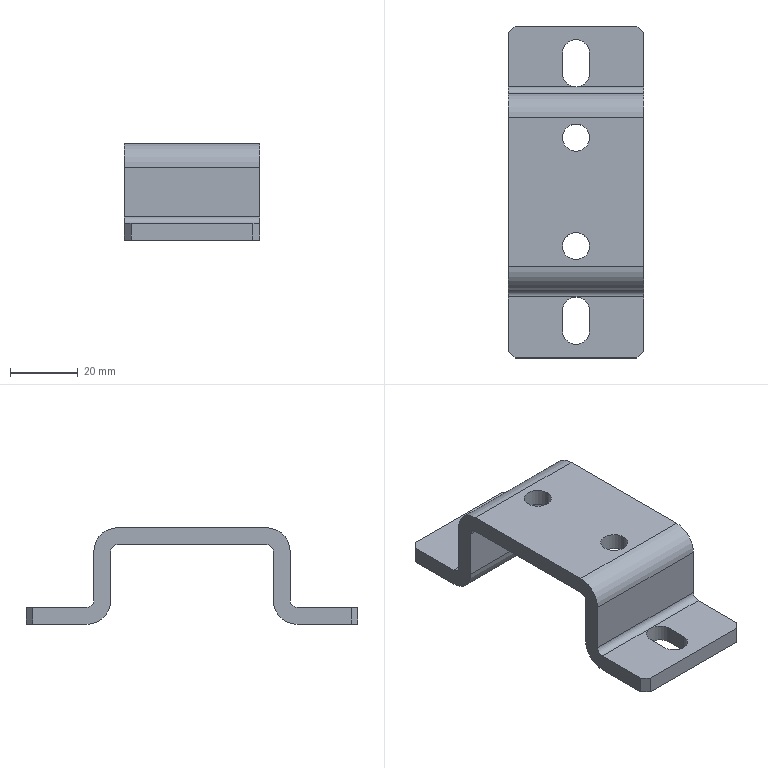Part | Creo | features DATUM PLANE 3, CURVE 2, ROUND 2, COORDINATE SYSTEM 1, CUT 1, PROTRUSION 1 | 1 solid | 38 faces | box 40 x 98 x 28.5 mm | volume 25930 mm3 | plane 22 | cylinder 16 | commonest cylinder face diameters 8 x8 4 x4 14 x4
STEP:
#1=CARTESIAN_POINT('',(0.,0.,0.));
#2=DIRECTION('',(0.,0.,1.));
#3=DIRECTION('',(1.,0.,0.));
#4=AXIS2_PLACEMENT_3D('',#1,#2,#3);
#5=CARTESIAN_POINT('',(4.,41.,0.));
#6=VERTEX_POINT('',#5);
#7=CARTESIAN_POINT('',(4.,35.,0.));
#8=VERTEX_POINT('',#7);
#9=CARTESIAN_POINT('',(4.,41.,0.));
#10=DIRECTION('',(0.,-1.,0.));
#11=VECTOR('',#10,6.);
#12=LINE('',#9,#11);
#13=EDGE_CURVE('',#6,#8,#12,.T.);
#14=ORIENTED_EDGE('',*,*,#13,.T.);
#15=CARTESIAN_POINT('',(0.,31.,0.));
#16=VERTEX_POINT('',#15);
#17=CARTESIAN_POINT('',(0.,35.,0.));
#18=DIRECTION('',(0.,0.,-1.));
#19=DIRECTION('',(1.,0.,0.));
#20=AXIS2_PLACEMENT_3D('',#17,#18,#19);
#21=CIRCLE('',#20,4.);
#22=EDGE_CURVE('',#8,#16,#21,.T.);
#23=ORIENTED_EDGE('',*,*,#22,.T.);
#24=CARTESIAN_POINT('',(20.,31.,0.));
#25=VERTEX_POINT('',#24);
#26=CARTESIAN_POINT('',(20.,31.,0.));
#27=DIRECTION('',(-1.,0.,0.));
#28=VECTOR('',#27,20.);
#29=LINE('',#26,#28);
#30=EDGE_CURVE('',#25,#16,#29,.T.);
#31=ORIENTED_EDGE('',*,*,#30,.F.);
#32=CARTESIAN_POINT('',(20.,47.,0.));
#33=VERTEX_POINT('',#32);
#34=CARTESIAN_POINT('',(20.,31.,0.));
#35=DIRECTION('',(0.,1.,0.));
#36=VECTOR('',#35,16.);
#37=LINE('',#34,#36);
#38=EDGE_CURVE('',#25,#33,#37,.T.);
#39=ORIENTED_EDGE('',*,*,#38,.T.);
#40=CARTESIAN_POINT('',(18.,49.,0.));
#41=VERTEX_POINT('',#40);
#42=CARTESIAN_POINT('',(20.,47.,0.));
#43=DIRECTION('',(-0.7071,0.7071,0.));
#44=VECTOR('',#43,2.828);
#45=LINE('',#42,#44);
#46=EDGE_CURVE('',#33,#41,#45,.T.);
#47=ORIENTED_EDGE('',*,*,#46,.T.);
#48=CARTESIAN_POINT('',(-18.,49.,0.));
#49=VERTEX_POINT('',#48);
#50=CARTESIAN_POINT('',(18.,49.,0.));
#51=DIRECTION('',(-1.,0.,0.));
#52=VECTOR('',#51,36.);
#53=LINE('',#50,#52);
#54=EDGE_CURVE('',#41,#49,#53,.T.);
#55=ORIENTED_EDGE('',*,*,#54,.T.);
#56=CARTESIAN_POINT('',(-20.,47.,0.));
#57=VERTEX_POINT('',#56);
#58=CARTESIAN_POINT('',(-18.,49.,0.));
#59=DIRECTION('',(-0.7071,-0.7071,0.));
#60=VECTOR('',#59,2.828);
#61=LINE('',#58,#60);
#62=EDGE_CURVE('',#49,#57,#61,.T.);
#63=ORIENTED_EDGE('',*,*,#62,.T.);
#64=CARTESIAN_POINT('',(-20.,31.,0.));
#65=VERTEX_POINT('',#64);
#66=CARTESIAN_POINT('',(-20.,47.,0.));
#67=DIRECTION('',(0.,-1.,0.));
#68=VECTOR('',#67,16.);
#69=LINE('',#66,#68);
#70=EDGE_CURVE('',#57,#65,#69,.T.);
#71=ORIENTED_EDGE('',*,*,#70,.T.);
#72=CARTESIAN_POINT('',(0.,31.,0.));
#73=DIRECTION('',(-1.,0.,0.));
#74=VECTOR('',#73,20.);
#75=LINE('',#72,#74);
#76=EDGE_CURVE('',#16,#65,#75,.T.);
#77=ORIENTED_EDGE('',*,*,#76,.F.);
#78=CARTESIAN_POINT('',(-4.,35.,0.));
#79=VERTEX_POINT('',#78);
#80=CARTESIAN_POINT('',(0.,35.,0.));
#81=DIRECTION('',(0.,0.,-1.));
#82=DIRECTION('',(0.,-1.,0.));
#83=AXIS2_PLACEMENT_3D('',#80,#81,#82);
#84=CIRCLE('',#83,4.);
#85=EDGE_CURVE('',#16,#79,#84,.T.);
#86=ORIENTED_EDGE('',*,*,#85,.T.);
#87=CARTESIAN_POINT('',(-4.,41.,0.));
#88=VERTEX_POINT('',#87);
#89=CARTESIAN_POINT('',(-4.,35.,0.));
#90=DIRECTION('',(0.,1.,0.));
#91=VECTOR('',#90,6.);
#92=LINE('',#89,#91);
#93=EDGE_CURVE('',#79,#88,#92,.T.);
#94=ORIENTED_EDGE('',*,*,#93,.T.);
#95=CARTESIAN_POINT('',(0.,41.,0.));
#96=DIRECTION('',(0.,0.,-1.));
#97=DIRECTION('',(-1.,0.,0.));
#98=AXIS2_PLACEMENT_3D('',#95,#96,#97);
#99=CIRCLE('',#98,4.);
#100=EDGE_CURVE('',#88,#6,#99,.T.);
#101=ORIENTED_EDGE('',*,*,#100,.T.);
#102=EDGE_LOOP('',(#14,#23,#31,#39,#47,#55,#63,#71,#77,#86,#94,#101));
#103=FACE_OUTER_BOUND('',#102,.F.);
#104=CARTESIAN_POINT('',(0.,0.,0.));
#105=DIRECTION('',(0.,0.,1.));
#106=DIRECTION('',(1.,0.,0.));
#107=AXIS2_PLACEMENT_3D('',#104,#105,#106);
#108=PLANE('',#107);
#109=ADVANCED_FACE('',(#103),#108,.F.);
#110=CARTESIAN_POINT('',(-4.,-41.,0.));
#111=VERTEX_POINT('',#110);
#112=CARTESIAN_POINT('',(-4.,-35.,0.));
#113=VERTEX_POINT('',#112);
#114=CARTESIAN_POINT('',(-4.,-41.,0.));
#115=DIRECTION('',(0.,1.,0.));
#116=VECTOR('',#115,6.);
#117=LINE('',#114,#116);
#118=EDGE_CURVE('',#111,#113,#117,.T.);
#119=ORIENTED_EDGE('',*,*,#118,.T.);
#120=CARTESIAN_POINT('',(0.,-31.,0.));
#121=VERTEX_POINT('',#120);
#122=CARTESIAN_POINT('',(0.,-35.,0.));
#123=DIRECTION('',(0.,0.,-1.));
#124=DIRECTION('',(-1.,0.,0.));
#125=AXIS2_PLACEMENT_3D('',#122,#123,#124);
#126=CIRCLE('',#125,4.);
#127=EDGE_CURVE('',#113,#121,#126,.T.);
#128=ORIENTED_EDGE('',*,*,#127,.T.);
#129=CARTESIAN_POINT('',(-20.,-31.,0.));
#130=VERTEX_POINT('',#129);
#131=CARTESIAN_POINT('',(-20.,-31.,0.));
#132=DIRECTION('',(1.,0.,0.));
#133=VECTOR('',#132,20.);
#134=LINE('',#131,#133);
#135=EDGE_CURVE('',#130,#121,#134,.T.);
#136=ORIENTED_EDGE('',*,*,#135,.F.);
#137=CARTESIAN_POINT('',(-20.,-47.,0.));
#138=VERTEX_POINT('',#137);
#139=CARTESIAN_POINT('',(-20.,-31.,0.));
#140=DIRECTION('',(0.,-1.,0.));
#141=VECTOR('',#140,16.);
#142=LINE('',#139,#141);
#143=EDGE_CURVE('',#130,#138,#142,.T.);
#144=ORIENTED_EDGE('',*,*,#143,.T.);
#145=CARTESIAN_POINT('',(-18.,-49.,0.));
#146=VERTEX_POINT('',#145);
#147=CARTESIAN_POINT('',(-20.,-47.,0.));
#148=DIRECTION('',(0.7071,-0.7071,0.));
#149=VECTOR('',#148,2.828);
#150=LINE('',#147,#149);
#151=EDGE_CURVE('',#138,#146,#150,.T.);
#152=ORIENTED_EDGE('',*,*,#151,.T.);
#153=CARTESIAN_POINT('',(18.,-49.,0.));
#154=VERTEX_POINT('',#153);
#155=CARTESIAN_POINT('',(-18.,-49.,0.));
#156=DIRECTION('',(1.,0.,0.));
#157=VECTOR('',#156,36.);
#158=LINE('',#155,#157);
#159=EDGE_CURVE('',#146,#154,#158,.T.);
#160=ORIENTED_EDGE('',*,*,#159,.T.);
#161=CARTESIAN_POINT('',(20.,-47.,0.));
#162=VERTEX_POINT('',#161);
#163=CARTESIAN_POINT('',(18.,-49.,0.));
#164=DIRECTION('',(0.7071,0.7071,0.));
#165=VECTOR('',#164,2.828);
#166=LINE('',#163,#165);
#167=EDGE_CURVE('',#154,#162,#166,.T.);
#168=ORIENTED_EDGE('',*,*,#167,.T.);
#169=CARTESIAN_POINT('',(20.,-31.,0.));
#170=VERTEX_POINT('',#169);
#171=CARTESIAN_POINT('',(20.,-47.,0.));
#172=DIRECTION('',(0.,1.,0.));
#173=VECTOR('',#172,16.);
#174=LINE('',#171,#173);
#175=EDGE_CURVE('',#162,#170,#174,.T.);
#176=ORIENTED_EDGE('',*,*,#175,.T.);
#177=CARTESIAN_POINT('',(0.,-31.,0.));
#178=DIRECTION('',(1.,0.,0.));
#179=VECTOR('',#178,20.);
#180=LINE('',#177,#179);
#181=EDGE_CURVE('',#121,#170,#180,.T.);
#182=ORIENTED_EDGE('',*,*,#181,.F.);
#183=CARTESIAN_POINT('',(4.,-35.,0.));
#184=VERTEX_POINT('',#183);
#185=CARTESIAN_POINT('',(0.,-35.,0.));
#186=DIRECTION('',(0.,0.,-1.));
#187=DIRECTION('',(0.,1.,0.));
#188=AXIS2_PLACEMENT_3D('',#185,#186,#187);
#189=CIRCLE('',#188,4.);
#190=EDGE_CURVE('',#121,#184,#189,.T.);
#191=ORIENTED_EDGE('',*,*,#190,.T.);
#192=CARTESIAN_POINT('',(4.,-41.,0.));
#193=VERTEX_POINT('',#192);
#194=CARTESIAN_POINT('',(4.,-35.,0.));
#195=DIRECTION('',(0.,-1.,0.));
#196=VECTOR('',#195,6.);
#197=LINE('',#194,#196);
#198=EDGE_CURVE('',#184,#193,#197,.T.);
#199=ORIENTED_EDGE('',*,*,#198,.T.);
#200=CARTESIAN_POINT('',(0.,-41.,0.));
#201=DIRECTION('',(0.,0.,-1.));
#202=DIRECTION('',(1.,0.,0.));
#203=AXIS2_PLACEMENT_3D('',#200,#201,#202);
#204=CIRCLE('',#203,4.);
#205=EDGE_CURVE('',#193,#111,#204,.T.);
#206=ORIENTED_EDGE('',*,*,#205,.T.);
#207=EDGE_LOOP('',(#119,#128,#136,#144,#152,#160,#168,#176,#182,#191,#199,#206));
#208=FACE_OUTER_BOUND('',#207,.F.);
#209=CARTESIAN_POINT('',(0.,0.,0.));
#210=DIRECTION('',(0.,0.,1.));
#211=DIRECTION('',(1.,0.,0.));
#212=AXIS2_PLACEMENT_3D('',#209,#210,#211);
#213=PLANE('',#212);
#214=ADVANCED_FACE('',(#208),#213,.F.);
#215=CARTESIAN_POINT('',(4.,41.,5.));
#216=VERTEX_POINT('',#215);
#217=CARTESIAN_POINT('',(4.,35.,5.));
#218=VERTEX_POINT('',#217);
#219=CARTESIAN_POINT('',(4.,41.,5.));
#220=DIRECTION('',(0.,-1.,0.));
#221=VECTOR('',#220,6.);
#222=LINE('',#219,#221);
#223=EDGE_CURVE('',#216,#218,#222,.T.);
#224=ORIENTED_EDGE('',*,*,#223,.T.);
#225=CARTESIAN_POINT('',(4.,35.,0.));
#226=DIRECTION('',(0.,0.,1.));
#227=VECTOR('',#226,5.);
#228=LINE('',#225,#227);
#229=EDGE_CURVE('',#8,#218,#228,.T.);
#230=ORIENTED_EDGE('',*,*,#229,.F.);
#231=ORIENTED_EDGE('',*,*,#13,.F.);
#232=CARTESIAN_POINT('',(4.,41.,0.));
#233=DIRECTION('',(0.,0.,1.));
#234=VECTOR('',#233,5.);
#235=LINE('',#232,#234);
#236=EDGE_CURVE('',#6,#216,#235,.T.);
#237=ORIENTED_EDGE('',*,*,#236,.T.);
#238=EDGE_LOOP('',(#224,#230,#231,#237));
#239=FACE_OUTER_BOUND('',#238,.F.);
#240=CARTESIAN_POINT('',(4.,41.,0.));
#241=DIRECTION('',(-1.,0.,0.));
#242=DIRECTION('',(0.,-1.,0.));
#243=AXIS2_PLACEMENT_3D('',#240,#241,#242);
#244=PLANE('',#243);
#245=ADVANCED_FACE('',(#239),#244,.T.);
#246=ORIENTED_EDGE('',*,*,#223,.F.);
#247=CARTESIAN_POINT('',(-4.,41.,5.));
#248=VERTEX_POINT('',#247);
#249=CARTESIAN_POINT('',(0.,41.,5.));
#250=DIRECTION('',(0.,0.,1.));
#251=DIRECTION('',(1.,0.,0.));
#252=AXIS2_PLACEMENT_3D('',#249,#250,#251);
#253=CIRCLE('',#252,4.);
#254=EDGE_CURVE('',#216,#248,#253,.T.);
#255=ORIENTED_EDGE('',*,*,#254,.T.);
#256=CARTESIAN_POINT('',(-4.,35.,5.));
#257=VERTEX_POINT('',#256);
#258=CARTESIAN_POINT('',(-4.,35.,5.));
#259=DIRECTION('',(0.,1.,0.));
#260=VECTOR('',#259,6.);
#261=LINE('',#258,#260);
#262=EDGE_CURVE('',#257,#248,#261,.T.);
#263=ORIENTED_EDGE('',*,*,#262,.F.);
#264=CARTESIAN_POINT('',(0.,31.,5.));
#265=VERTEX_POINT('',#264);
#266=CARTESIAN_POINT('',(0.,35.,5.));
#267=DIRECTION('',(0.,0.,1.));
#268=DIRECTION('',(-1.,0.,0.));
#269=AXIS2_PLACEMENT_3D('',#266,#267,#268);
#270=CIRCLE('',#269,4.);
#271=EDGE_CURVE('',#257,#265,#270,.T.);
#272=ORIENTED_EDGE('',*,*,#271,.T.);
#273=CARTESIAN_POINT('',(-20.,31.,5.));
#274=VERTEX_POINT('',#273);
#275=CARTESIAN_POINT('',(0.,31.,5.));
#276=DIRECTION('',(-1.,0.,0.));
#277=VECTOR('',#276,20.);
#278=LINE('',#275,#277);
#279=EDGE_CURVE('',#265,#274,#278,.T.);
#280=ORIENTED_EDGE('',*,*,#279,.T.);
#281=CARTESIAN_POINT('',(-20.,47.,5.));
#282=VERTEX_POINT('',#281);
#283=CARTESIAN_POINT('',(-20.,47.,5.));
#284=DIRECTION('',(0.,-1.,0.));
#285=VECTOR('',#284,16.);
#286=LINE('',#283,#285);
#287=EDGE_CURVE('',#282,#274,#286,.T.);
#288=ORIENTED_EDGE('',*,*,#287,.F.);
#289=CARTESIAN_POINT('',(-18.,49.,5.));
#290=VERTEX_POINT('',#289);
#291=CARTESIAN_POINT('',(-18.,49.,5.));
#292=DIRECTION('',(-0.7071,-0.7071,0.));
#293=VECTOR('',#292,2.828);
#294=LINE('',#291,#293);
#295=EDGE_CURVE('',#290,#282,#294,.T.);
#296=ORIENTED_EDGE('',*,*,#295,.F.);
#297=CARTESIAN_POINT('',(18.,49.,5.));
#298=VERTEX_POINT('',#297);
#299=CARTESIAN_POINT('',(18.,49.,5.));
#300=DIRECTION('',(-1.,0.,0.));
#301=VECTOR('',#300,36.);
#302=LINE('',#299,#301);
#303=EDGE_CURVE('',#298,#290,#302,.T.);
#304=ORIENTED_EDGE('',*,*,#303,.F.);
#305=CARTESIAN_POINT('',(20.,47.,5.));
#306=VERTEX_POINT('',#305);
#307=CARTESIAN_POINT('',(20.,47.,5.));
#308=DIRECTION('',(-0.7071,0.7071,0.));
#309=VECTOR('',#308,2.828);
#310=LINE('',#307,#309);
#311=EDGE_CURVE('',#306,#298,#310,.T.);
#312=ORIENTED_EDGE('',*,*,#311,.F.);
#313=CARTESIAN_POINT('',(20.,31.,5.));
#314=VERTEX_POINT('',#313);
#315=CARTESIAN_POINT('',(20.,47.,5.));
#316=DIRECTION('',(0.,-1.,0.));
#317=VECTOR('',#316,16.);
#318=LINE('',#315,#317);
#319=EDGE_CURVE('',#306,#314,#318,.T.);
#320=ORIENTED_EDGE('',*,*,#319,.T.);
#321=CARTESIAN_POINT('',(20.,31.,5.));
#322=DIRECTION('',(-1.,0.,0.));
#323=VECTOR('',#322,20.);
#324=LINE('',#321,#323);
#325=EDGE_CURVE('',#314,#265,#324,.T.);
#326=ORIENTED_EDGE('',*,*,#325,.T.);
#327=CARTESIAN_POINT('',(0.,35.,5.));
#328=DIRECTION('',(0.,0.,1.));
#329=DIRECTION('',(0.,-1.,0.));
#330=AXIS2_PLACEMENT_3D('',#327,#328,#329);
#331=CIRCLE('',#330,4.);
#332=EDGE_CURVE('',#265,#218,#331,.T.);
#333=ORIENTED_EDGE('',*,*,#332,.T.);
#334=EDGE_LOOP('',(#246,#255,#263,#272,#280,#288,#296,#304,#312,#320,#326,#333));
#335=FACE_OUTER_BOUND('',#334,.F.);
#336=CARTESIAN_POINT('',(20.,29.,5.));
#337=DIRECTION('',(0.,0.,-1.));
#338=DIRECTION('',(0.,1.,0.));
#339=AXIS2_PLACEMENT_3D('',#336,#337,#338);
#340=PLANE('',#339);
#341=ADVANCED_FACE('',(#335),#340,.F.);
#342=ORIENTED_EDGE('',*,*,#254,.F.);
#343=ORIENTED_EDGE('',*,*,#236,.F.);
#344=ORIENTED_EDGE('',*,*,#100,.F.);
#345=CARTESIAN_POINT('',(-4.,41.,0.));
#346=DIRECTION('',(0.,0.,1.));
#347=VECTOR('',#346,5.);
#348=LINE('',#345,#347);
#349=EDGE_CURVE('',#88,#248,#348,.T.);
#350=ORIENTED_EDGE('',*,*,#349,.T.);
#351=EDGE_LOOP('',(#342,#343,#344,#350));
#352=FACE_OUTER_BOUND('',#351,.F.);
#353=CARTESIAN_POINT('',(0.,41.,0.));
#354=DIRECTION('',(0.,0.,1.));
#355=DIRECTION('',(1.,0.,0.));
#356=AXIS2_PLACEMENT_3D('',#353,#354,#355);
#357=CYLINDRICAL_SURFACE('',#356,4.);
#358=ADVANCED_FACE('',(#352),#357,.F.);
#359=ORIENTED_EDGE('',*,*,#262,.T.);
#360=ORIENTED_EDGE('',*,*,#349,.F.);
#361=ORIENTED_EDGE('',*,*,#93,.F.);
#362=CARTESIAN_POINT('',(-4.,35.,0.));
#363=DIRECTION('',(0.,0.,1.));
#364=VECTOR('',#363,5.);
#365=LINE('',#362,#364);
#366=EDGE_CURVE('',#79,#257,#365,.T.);
#367=ORIENTED_EDGE('',*,*,#366,.T.);
#368=EDGE_LOOP('',(#359,#360,#361,#367));
#369=FACE_OUTER_BOUND('',#368,.F.);
#370=CARTESIAN_POINT('',(-4.,35.,0.));
#371=DIRECTION('',(1.,0.,0.));
#372=DIRECTION('',(0.,1.,0.));
#373=AXIS2_PLACEMENT_3D('',#370,#371,#372);
#374=PLANE('',#373);
#375=ADVANCED_FACE('',(#369),#374,.T.);
#376=ORIENTED_EDGE('',*,*,#271,.F.);
#377=ORIENTED_EDGE('',*,*,#366,.F.);
#378=ORIENTED_EDGE('',*,*,#85,.F.);
#379=ORIENTED_EDGE('',*,*,#22,.F.);
#380=ORIENTED_EDGE('',*,*,#229,.T.);
#381=ORIENTED_EDGE('',*,*,#332,.F.);
#382=EDGE_LOOP('',(#376,#377,#378,#379,#380,#381));
#383=FACE_OUTER_BOUND('',#382,.F.);
#384=CARTESIAN_POINT('',(0.,35.,0.));
#385=DIRECTION('',(0.,0.,1.));
#386=DIRECTION('',(1.,0.,0.));
#387=AXIS2_PLACEMENT_3D('',#384,#385,#386);
#388=CYLINDRICAL_SURFACE('',#387,4.);
#389=ADVANCED_FACE('',(#383),#388,.F.);
#390=ORIENTED_EDGE('',*,*,#325,.F.);
#391=CARTESIAN_POINT('',(20.,29.,7.));
#392=VERTEX_POINT('',#391);
#393=CARTESIAN_POINT('',(20.,31.,7.));
#394=DIRECTION('',(-1.,0.,0.));
#395=DIRECTION('',(0.,0.,-1.));
#396=AXIS2_PLACEMENT_3D('',#393,#394,#395);
#397=CIRCLE('',#396,2.);
#398=EDGE_CURVE('',#314,#392,#397,.T.);
#399=ORIENTED_EDGE('',*,*,#398,.T.);
#400=CARTESIAN_POINT('',(-20.,29.,7.));
#401=VERTEX_POINT('',#400);
#402=CARTESIAN_POINT('',(20.,29.,7.));
#403=DIRECTION('',(-1.,0.,0.));
#404=VECTOR('',#403,40.);
#405=LINE('',#402,#404);
#406=EDGE_CURVE('',#392,#401,#405,.T.);
#407=ORIENTED_EDGE('',*,*,#406,.T.);
#408=CARTESIAN_POINT('',(-20.,31.,7.));
#409=DIRECTION('',(1.,0.,0.));
#410=DIRECTION('',(0.,-1.,0.));
#411=AXIS2_PLACEMENT_3D('',#408,#409,#410);
#412=CIRCLE('',#411,2.);
#413=EDGE_CURVE('',#401,#274,#412,.T.);
#414=ORIENTED_EDGE('',*,*,#413,.T.);
#415=ORIENTED_EDGE('',*,*,#279,.F.);
#416=EDGE_LOOP('',(#390,#399,#407,#414,#415));
#417=FACE_OUTER_BOUND('',#416,.F.);
#418=CARTESIAN_POINT('',(72.144,31.,7.));
#419=DIRECTION('',(-1.,0.,0.));
#420=DIRECTION('',(0.,0.,-1.));
#421=AXIS2_PLACEMENT_3D('',#418,#419,#420);
#422=CYLINDRICAL_SURFACE('',#421,2.);
#423=ADVANCED_FACE('',(#417),#422,.F.);
#424=CARTESIAN_POINT('',(20.,-22.,28.5));
#425=VERTEX_POINT('',#424);
#426=CARTESIAN_POINT('',(20.,-29.,21.5));
#427=VERTEX_POINT('',#426);
#428=CARTESIAN_POINT('',(20.,-22.,21.5));
#429=DIRECTION('',(1.,0.,0.));
#430=DIRECTION('',(0.,0.,1.));
#431=AXIS2_PLACEMENT_3D('',#428,#429,#430);
#432=CIRCLE('',#431,7.);
#433=EDGE_CURVE('',#425,#427,#432,.T.);
#434=ORIENTED_EDGE('',*,*,#433,.F.);
#435=CARTESIAN_POINT('',(20.,22.,28.5));
#436=VERTEX_POINT('',#435);
#437=CARTESIAN_POINT('',(20.,-22.,28.5));
#438=DIRECTION('',(0.,1.,0.));
#439=VECTOR('',#438,44.);
#440=LINE('',#437,#439);
#441=EDGE_CURVE('',#425,#436,#440,.T.);
#442=ORIENTED_EDGE('',*,*,#441,.T.);
#443=CARTESIAN_POINT('',(20.,29.,21.5));
#444=VERTEX_POINT('',#443);
#445=CARTESIAN_POINT('',(20.,22.,21.5));
#446=DIRECTION('',(1.,0.,0.));
#447=DIRECTION('',(0.,1.,0.));
#448=AXIS2_PLACEMENT_3D('',#445,#446,#447);
#449=CIRCLE('',#448,7.);
#450=EDGE_CURVE('',#444,#436,#449,.T.);
#451=ORIENTED_EDGE('',*,*,#450,.F.);
#452=CARTESIAN_POINT('',(20.,29.,21.5));
#453=DIRECTION('',(0.,0.,-1.));
#454=VECTOR('',#453,14.5);
#455=LINE('',#452,#454);
#456=EDGE_CURVE('',#444,#392,#455,.T.);
#457=ORIENTED_EDGE('',*,*,#456,.T.);
#458=ORIENTED_EDGE('',*,*,#398,.F.);
#459=ORIENTED_EDGE('',*,*,#319,.F.);
#460=CARTESIAN_POINT('',(20.,47.,0.));
#461=DIRECTION('',(0.,0.,1.));
#462=VECTOR('',#461,5.);
#463=LINE('',#460,#462);
#464=EDGE_CURVE('',#33,#306,#463,.T.);
#465=ORIENTED_EDGE('',*,*,#464,.F.);
#466=ORIENTED_EDGE('',*,*,#38,.F.);
#467=CARTESIAN_POINT('',(20.,24.,7.));
#468=VERTEX_POINT('',#467);
#469=CARTESIAN_POINT('',(20.,31.,7.));
#470=DIRECTION('',(1.,0.,0.));
#471=DIRECTION('',(0.,-1.,0.));
#472=AXIS2_PLACEMENT_3D('',#469,#470,#471);
#473=CIRCLE('',#472,7.);
#474=EDGE_CURVE('',#468,#25,#473,.T.);
#475=ORIENTED_EDGE('',*,*,#474,.F.);
#476=CARTESIAN_POINT('',(20.,24.,21.5));
#477=VERTEX_POINT('',#476);
#478=CARTESIAN_POINT('',(20.,24.,7.));
#479=DIRECTION('',(0.,0.,1.));
#480=VECTOR('',#479,14.5);
#481=LINE('',#478,#480);
#482=EDGE_CURVE('',#468,#477,#481,.T.);
#483=ORIENTED_EDGE('',*,*,#482,.T.);
#484=CARTESIAN_POINT('',(20.,22.,23.5));
#485=VERTEX_POINT('',#484);
#486=CARTESIAN_POINT('',(20.,22.,21.5));
#487=DIRECTION('',(-1.,0.,0.));
#488=DIRECTION('',(0.,0.,1.));
#489=AXIS2_PLACEMENT_3D('',#486,#487,#488);
#490=CIRCLE('',#489,2.);
#491=EDGE_CURVE('',#485,#477,#490,.T.);
#492=ORIENTED_EDGE('',*,*,#491,.F.);
#493=CARTESIAN_POINT('',(20.,-22.,23.5));
#494=VERTEX_POINT('',#493);
#495=CARTESIAN_POINT('',(20.,22.,23.5));
#496=DIRECTION('',(0.,-1.,0.));
#497=VECTOR('',#496,44.);
#498=LINE('',#495,#497);
#499=EDGE_CURVE('',#485,#494,#498,.T.);
#500=ORIENTED_EDGE('',*,*,#499,.T.);
#501=CARTESIAN_POINT('',(20.,-24.,21.5));
#502=VERTEX_POINT('',#501);
#503=CARTESIAN_POINT('',(20.,-22.,21.5));
#504=DIRECTION('',(-1.,0.,0.));
#505=DIRECTION('',(0.,-1.,0.));
#506=AXIS2_PLACEMENT_3D('',#503,#504,#505);
#507=CIRCLE('',#506,2.);
#508=EDGE_CURVE('',#502,#494,#507,.T.);
#509=ORIENTED_EDGE('',*,*,#508,.F.);
#510=CARTESIAN_POINT('',(20.,-24.,7.));
#511=VERTEX_POINT('',#510);
#512=CARTESIAN_POINT('',(20.,-24.,7.));
#513=DIRECTION('',(0.,0.,1.));
#514=VECTOR('',#513,14.5);
#515=LINE('',#512,#514);
#516=EDGE_CURVE('',#511,#502,#515,.T.);
#517=ORIENTED_EDGE('',*,*,#516,.F.);
#518=CARTESIAN_POINT('',(20.,-31.,7.));
#519=DIRECTION('',(1.,0.,0.));
#520=DIRECTION('',(0.,0.,-1.));
#521=AXIS2_PLACEMENT_3D('',#518,#519,#520);
#522=CIRCLE('',#521,7.);
#523=EDGE_CURVE('',#170,#511,#522,.T.);
#524=ORIENTED_EDGE('',*,*,#523,.F.);
#525=ORIENTED_EDGE('',*,*,#175,.F.);
#526=CARTESIAN_POINT('',(20.,-47.,5.));
#527=VERTEX_POINT('',#526);
#528=CARTESIAN_POINT('',(20.,-47.,0.));
#529=DIRECTION('',(0.,0.,1.));
#530=VECTOR('',#529,5.);
#531=LINE('',#528,#530);
#532=EDGE_CURVE('',#162,#527,#531,.T.);
#533=ORIENTED_EDGE('',*,*,#532,.T.);
#534=CARTESIAN_POINT('',(20.,-31.,5.));
#535=VERTEX_POINT('',#534);
#536=CARTESIAN_POINT('',(20.,-47.,5.));
#537=DIRECTION('',(0.,1.,0.));
#538=VECTOR('',#537,16.);
#539=LINE('',#536,#538);
#540=EDGE_CURVE('',#527,#535,#539,.T.);
#541=ORIENTED_EDGE('',*,*,#540,.T.);
#542=CARTESIAN_POINT('',(20.,-29.,7.));
#543=VERTEX_POINT('',#542);
#544=CARTESIAN_POINT('',(20.,-31.,7.));
#545=DIRECTION('',(-1.,0.,0.));
#546=DIRECTION('',(0.,1.,0.));
#547=AXIS2_PLACEMENT_3D('',#544,#545,#546);
#548=CIRCLE('',#547,2.);
#549=EDGE_CURVE('',#543,#535,#548,.T.);
#550=ORIENTED_EDGE('',*,*,#549,.F.);
#551=CARTESIAN_POINT('',(20.,-29.,21.5));
#552=DIRECTION('',(0.,0.,-1.));
#553=VECTOR('',#552,14.5);
#554=LINE('',#551,#553);
#555=EDGE_CURVE('',#427,#543,#554,.T.);
#556=ORIENTED_EDGE('',*,*,#555,.F.);
#557=EDGE_LOOP('',(#434,#442,#451,#457,#458,#459,#465,#466,#475,#483,#492,#500,#509,#517,#524,#525,#533,#541,#550,#556));
#558=FACE_OUTER_BOUND('',#557,.F.);
#559=CARTESIAN_POINT('',(20.,-47.,0.));
#560=DIRECTION('',(1.,0.,0.));
#561=DIRECTION('',(0.,1.,0.));
#562=AXIS2_PLACEMENT_3D('',#559,#560,#561);
#563=PLANE('',#562);
#564=ADVANCED_FACE('',(#558),#563,.T.);
#565=ORIENTED_EDGE('',*,*,#433,.T.);
#566=CARTESIAN_POINT('',(-20.,-29.,21.5));
#567=VERTEX_POINT('',#566);
#568=CARTESIAN_POINT('',(-20.,-29.,21.5));
#569=DIRECTION('',(1.,0.,0.));
#570=VECTOR('',#569,40.);
#571=LINE('',#568,#570);
#572=EDGE_CURVE('',#567,#427,#571,.T.);
#573=ORIENTED_EDGE('',*,*,#572,.F.);
#574=CARTESIAN_POINT('',(-20.,-22.,28.5));
#575=VERTEX_POINT('',#574);
#576=CARTESIAN_POINT('',(-20.,-22.,21.5));
#577=DIRECTION('',(-1.,0.,0.));
#578=DIRECTION('',(0.,-1.,0.));
#579=AXIS2_PLACEMENT_3D('',#576,#577,#578);
#580=CIRCLE('',#579,7.);
#581=EDGE_CURVE('',#567,#575,#580,.T.);
#582=ORIENTED_EDGE('',*,*,#581,.T.);
#583=CARTESIAN_POINT('',(-20.,-22.,28.5));
#584=DIRECTION('',(1.,0.,0.));
#585=VECTOR('',#584,40.);
#586=LINE('',#583,#585);
#587=EDGE_CURVE('',#575,#425,#586,.T.);
#588=ORIENTED_EDGE('',*,*,#587,.T.);
#589=EDGE_LOOP('',(#565,#573,#582,#588));
#590=FACE_OUTER_BOUND('',#589,.F.);
#591=CARTESIAN_POINT('',(-72.144,-22.,21.5));
#592=DIRECTION('',(1.,0.,0.));
#593=DIRECTION('',(0.,0.,1.));
#594=AXIS2_PLACEMENT_3D('',#591,#592,#593);
#595=CYLINDRICAL_SURFACE('',#594,7.);
#596=ADVANCED_FACE('',(#590),#595,.T.);
#597=ORIENTED_EDGE('',*,*,#572,.T.);
#598=ORIENTED_EDGE('',*,*,#555,.T.);
#599=CARTESIAN_POINT('',(-20.,-29.,7.));
#600=VERTEX_POINT('',#599);
#601=CARTESIAN_POINT('',(20.,-29.,7.));
#602=DIRECTION('',(-1.,0.,0.));
#603=VECTOR('',#602,40.);
#604=LINE('',#601,#603);
#605=EDGE_CURVE('',#543,#600,#604,.T.);
#606=ORIENTED_EDGE('',*,*,#605,.T.);
#607=CARTESIAN_POINT('',(-20.,-29.,21.5));
#608=DIRECTION('',(0.,0.,-1.));
#609=VECTOR('',#608,14.5);
#610=LINE('',#607,#609);
#611=EDGE_CURVE('',#567,#600,#610,.T.);
#612=ORIENTED_EDGE('',*,*,#611,.F.);
#613=EDGE_LOOP('',(#597,#598,#606,#612));
#614=FACE_OUTER_BOUND('',#613,.F.);
#615=CARTESIAN_POINT('',(20.,-29.,5.));
#616=DIRECTION('',(0.,1.,0.));
#617=DIRECTION('',(0.,0.,1.));
#618=AXIS2_PLACEMENT_3D('',#615,#616,#617);
#619=PLANE('',#618);
#620=ADVANCED_FACE('',(#614),#619,.F.);
#621=ORIENTED_EDGE('',*,*,#605,.F.);
#622=ORIENTED_EDGE('',*,*,#549,.T.);
#623=CARTESIAN_POINT('',(0.,-31.,5.));
#624=VERTEX_POINT('',#623);
#625=CARTESIAN_POINT('',(20.,-31.,5.));
#626=DIRECTION('',(-1.,0.,0.));
#627=VECTOR('',#626,20.);
#628=LINE('',#625,#627);
#629=EDGE_CURVE('',#535,#624,#628,.T.);
#630=ORIENTED_EDGE('',*,*,#629,.T.);
#631=CARTESIAN_POINT('',(-20.,-31.,5.));
#632=VERTEX_POINT('',#631);
#633=CARTESIAN_POINT('',(0.,-31.,5.));
#634=DIRECTION('',(-1.,0.,0.));
#635=VECTOR('',#634,20.);
#636=LINE('',#633,#635);
#637=EDGE_CURVE('',#624,#632,#636,.T.);
#638=ORIENTED_EDGE('',*,*,#637,.T.);
#639=CARTESIAN_POINT('',(-20.,-31.,7.));
#640=DIRECTION('',(1.,0.,0.));
#641=DIRECTION('',(0.,0.,-1.));
#642=AXIS2_PLACEMENT_3D('',#639,#640,#641);
#643=CIRCLE('',#642,2.);
#644=EDGE_CURVE('',#632,#600,#643,.T.);
#645=ORIENTED_EDGE('',*,*,#644,.T.);
#646=EDGE_LOOP('',(#621,#622,#630,#638,#645));
#647=FACE_OUTER_BOUND('',#646,.F.);
#648=CARTESIAN_POINT('',(72.144,-31.,7.));
#649=DIRECTION('',(-1.,0.,0.));
#650=DIRECTION('',(0.,1.,0.));
#651=AXIS2_PLACEMENT_3D('',#648,#649,#650);
#652=CYLINDRICAL_SURFACE('',#651,2.);
#653=ADVANCED_FACE('',(#647),#652,.F.);
#654=CARTESIAN_POINT('',(-4.,-41.,5.));
#655=VERTEX_POINT('',#654);
#656=CARTESIAN_POINT('',(-4.,-35.,5.));
#657=VERTEX_POINT('',#656);
#658=CARTESIAN_POINT('',(-4.,-41.,5.));
#659=DIRECTION('',(0.,1.,0.));
#660=VECTOR('',#659,6.);
#661=LINE('',#658,#660);
#662=EDGE_CURVE('',#655,#657,#661,.T.);
#663=ORIENTED_EDGE('',*,*,#662,.F.);
#664=CARTESIAN_POINT('',(4.,-41.,5.));
#665=VERTEX_POINT('',#664);
#666=CARTESIAN_POINT('',(0.,-41.,5.));
#667=DIRECTION('',(0.,0.,1.));
#668=DIRECTION('',(-1.,0.,0.));
#669=AXIS2_PLACEMENT_3D('',#666,#667,#668);
#670=CIRCLE('',#669,4.);
#671=EDGE_CURVE('',#655,#665,#670,.T.);
#672=ORIENTED_EDGE('',*,*,#671,.T.);
#673=CARTESIAN_POINT('',(4.,-35.,5.));
#674=VERTEX_POINT('',#673);
#675=CARTESIAN_POINT('',(4.,-35.,5.));
#676=DIRECTION('',(0.,-1.,0.));
#677=VECTOR('',#676,6.);
#678=LINE('',#675,#677);
#679=EDGE_CURVE('',#674,#665,#678,.T.);
#680=ORIENTED_EDGE('',*,*,#679,.F.);
#681=CARTESIAN_POINT('',(0.,-35.,5.));
#682=DIRECTION('',(0.,0.,1.));
#683=DIRECTION('',(1.,0.,0.));
#684=AXIS2_PLACEMENT_3D('',#681,#682,#683);
#685=CIRCLE('',#684,4.);
#686=EDGE_CURVE('',#674,#624,#685,.T.);
#687=ORIENTED_EDGE('',*,*,#686,.T.);
#688=ORIENTED_EDGE('',*,*,#629,.F.);
#689=ORIENTED_EDGE('',*,*,#540,.F.);
#690=CARTESIAN_POINT('',(18.,-49.,5.));
#691=VERTEX_POINT('',#690);
#692=CARTESIAN_POINT('',(18.,-49.,5.));
#693=DIRECTION('',(0.7071,0.7071,0.));
#694=VECTOR('',#693,2.828);
#695=LINE('',#692,#694);
#696=EDGE_CURVE('',#691,#527,#695,.T.);
#697=ORIENTED_EDGE('',*,*,#696,.F.);
#698=CARTESIAN_POINT('',(-18.,-49.,5.));
#699=VERTEX_POINT('',#698);
#700=CARTESIAN_POINT('',(-18.,-49.,5.));
#701=DIRECTION('',(1.,0.,0.));
#702=VECTOR('',#701,36.);
#703=LINE('',#700,#702);
#704=EDGE_CURVE('',#699,#691,#703,.T.);
#705=ORIENTED_EDGE('',*,*,#704,.F.);
#706=CARTESIAN_POINT('',(-20.,-47.,5.));
#707=VERTEX_POINT('',#706);
#708=CARTESIAN_POINT('',(-20.,-47.,5.));
#709=DIRECTION('',(0.7071,-0.7071,0.));
#710=VECTOR('',#709,2.828);
#711=LINE('',#708,#710);
#712=EDGE_CURVE('',#707,#699,#711,.T.);
#713=ORIENTED_EDGE('',*,*,#712,.F.);
#714=CARTESIAN_POINT('',(-20.,-47.,5.));
#715=DIRECTION('',(0.,1.,0.));
#716=VECTOR('',#715,16.);
#717=LINE('',#714,#716);
#718=EDGE_CURVE('',#707,#632,#717,.T.);
#719=ORIENTED_EDGE('',*,*,#718,.T.);
#720=ORIENTED_EDGE('',*,*,#637,.F.);
#721=CARTESIAN_POINT('',(0.,-35.,5.));
#722=DIRECTION('',(0.,0.,1.));
#723=DIRECTION('',(0.,1.,0.));
#724=AXIS2_PLACEMENT_3D('',#721,#722,#723);
#725=CIRCLE('',#724,4.);
#726=EDGE_CURVE('',#624,#657,#725,.T.);
#727=ORIENTED_EDGE('',*,*,#726,.T.);
#728=EDGE_LOOP('',(#663,#672,#680,#687,#688,#689,#697,#705,#713,#719,#720,#727));
#729=FACE_OUTER_BOUND('',#728,.F.);
#730=CARTESIAN_POINT('',(20.,-49.,5.));
#731=DIRECTION('',(0.,0.,-1.));
#732=DIRECTION('',(0.,1.,0.));
#733=AXIS2_PLACEMENT_3D('',#730,#731,#732);
#734=PLANE('',#733);
#735=ADVANCED_FACE('',(#729),#734,.F.);
#736=ORIENTED_EDGE('',*,*,#662,.T.);
#737=CARTESIAN_POINT('',(-4.,-35.,0.));
#738=DIRECTION('',(0.,0.,1.));
#739=VECTOR('',#738,5.);
#740=LINE('',#737,#739);
#741=EDGE_CURVE('',#113,#657,#740,.T.);
#742=ORIENTED_EDGE('',*,*,#741,.F.);
#743=ORIENTED_EDGE('',*,*,#118,.F.);
#744=CARTESIAN_POINT('',(-4.,-41.,0.));
#745=DIRECTION('',(0.,0.,1.));
#746=VECTOR('',#745,5.);
#747=LINE('',#744,#746);
#748=EDGE_CURVE('',#111,#655,#747,.T.);
#749=ORIENTED_EDGE('',*,*,#748,.T.);
#750=EDGE_LOOP('',(#736,#742,#743,#749));
#751=FACE_OUTER_BOUND('',#750,.F.);
#752=CARTESIAN_POINT('',(-4.,-41.,0.));
#753=DIRECTION('',(1.,0.,0.));
#754=DIRECTION('',(0.,1.,0.));
#755=AXIS2_PLACEMENT_3D('',#752,#753,#754);
#756=PLANE('',#755);
#757=ADVANCED_FACE('',(#751),#756,.T.);
#758=ORIENTED_EDGE('',*,*,#686,.F.);
#759=CARTESIAN_POINT('',(4.,-35.,0.));
#760=DIRECTION('',(0.,0.,1.));
#761=VECTOR('',#760,5.);
#762=LINE('',#759,#761);
#763=EDGE_CURVE('',#184,#674,#762,.T.);
#764=ORIENTED_EDGE('',*,*,#763,.F.);
#765=ORIENTED_EDGE('',*,*,#190,.F.);
#766=ORIENTED_EDGE('',*,*,#127,.F.);
#767=ORIENTED_EDGE('',*,*,#741,.T.);
#768=ORIENTED_EDGE('',*,*,#726,.F.);
#769=EDGE_LOOP('',(#758,#764,#765,#766,#767,#768));
#770=FACE_OUTER_BOUND('',#769,.F.);
#771=CARTESIAN_POINT('',(0.,-35.,0.));
#772=DIRECTION('',(0.,0.,1.));
#773=DIRECTION('',(1.,0.,0.));
#774=AXIS2_PLACEMENT_3D('',#771,#772,#773);
#775=CYLINDRICAL_SURFACE('',#774,4.);
#776=ADVANCED_FACE('',(#770),#775,.F.);
#777=ORIENTED_EDGE('',*,*,#679,.T.);
#778=CARTESIAN_POINT('',(4.,-41.,0.));
#779=DIRECTION('',(0.,0.,1.));
#780=VECTOR('',#779,5.);
#781=LINE('',#778,#780);
#782=EDGE_CURVE('',#193,#665,#781,.T.);
#783=ORIENTED_EDGE('',*,*,#782,.F.);
#784=ORIENTED_EDGE('',*,*,#198,.F.);
#785=ORIENTED_EDGE('',*,*,#763,.T.);
#786=EDGE_LOOP('',(#777,#783,#784,#785));
#787=FACE_OUTER_BOUND('',#786,.F.);
#788=CARTESIAN_POINT('',(4.,-35.,0.));
#789=DIRECTION('',(-1.,0.,0.));
#790=DIRECTION('',(0.,-1.,0.));
#791=AXIS2_PLACEMENT_3D('',#788,#789,#790);
#792=PLANE('',#791);
#793=ADVANCED_FACE('',(#787),#792,.T.);
#794=ORIENTED_EDGE('',*,*,#671,.F.);
#795=ORIENTED_EDGE('',*,*,#748,.F.);
#796=ORIENTED_EDGE('',*,*,#205,.F.);
#797=ORIENTED_EDGE('',*,*,#782,.T.);
#798=EDGE_LOOP('',(#794,#795,#796,#797));
#799=FACE_OUTER_BOUND('',#798,.F.);
#800=CARTESIAN_POINT('',(0.,-41.,0.));
#801=DIRECTION('',(0.,0.,1.));
#802=DIRECTION('',(1.,0.,0.));
#803=AXIS2_PLACEMENT_3D('',#800,#801,#802);
#804=CYLINDRICAL_SURFACE('',#803,4.);
#805=ADVANCED_FACE('',(#799),#804,.F.);
#806=ORIENTED_EDGE('',*,*,#696,.T.);
#807=ORIENTED_EDGE('',*,*,#532,.F.);
#808=ORIENTED_EDGE('',*,*,#167,.F.);
#809=CARTESIAN_POINT('',(18.,-49.,0.));
#810=DIRECTION('',(0.,0.,1.));
#811=VECTOR('',#810,5.);
#812=LINE('',#809,#811);
#813=EDGE_CURVE('',#154,#691,#812,.T.);
#814=ORIENTED_EDGE('',*,*,#813,.T.);
#815=EDGE_LOOP('',(#806,#807,#808,#814));
#816=FACE_OUTER_BOUND('',#815,.F.);
#817=CARTESIAN_POINT('',(18.,-49.,0.));
#818=DIRECTION('',(0.7071,-0.7071,0.));
#819=DIRECTION('',(0.7071,0.7071,0.));
#820=AXIS2_PLACEMENT_3D('',#817,#818,#819);
#821=PLANE('',#820);
#822=ADVANCED_FACE('',(#816),#821,.T.);
#823=ORIENTED_EDGE('',*,*,#704,.T.);
#824=ORIENTED_EDGE('',*,*,#813,.F.);
#825=ORIENTED_EDGE('',*,*,#159,.F.);
#826=CARTESIAN_POINT('',(-18.,-49.,0.));
#827=DIRECTION('',(0.,0.,1.));
#828=VECTOR('',#827,5.);
#829=LINE('',#826,#828);
#830=EDGE_CURVE('',#146,#699,#829,.T.);
#831=ORIENTED_EDGE('',*,*,#830,.T.);
#832=EDGE_LOOP('',(#823,#824,#825,#831));
#833=FACE_OUTER_BOUND('',#832,.F.);
#834=CARTESIAN_POINT('',(-18.,-49.,0.));
#835=DIRECTION('',(0.,-1.,0.));
#836=DIRECTION('',(1.,0.,0.));
#837=AXIS2_PLACEMENT_3D('',#834,#835,#836);
#838=PLANE('',#837);
#839=ADVANCED_FACE('',(#833),#838,.T.);
#840=ORIENTED_EDGE('',*,*,#712,.T.);
#841=ORIENTED_EDGE('',*,*,#830,.F.);
#842=ORIENTED_EDGE('',*,*,#151,.F.);
#843=CARTESIAN_POINT('',(-20.,-47.,0.));
#844=DIRECTION('',(0.,0.,1.));
#845=VECTOR('',#844,5.);
#846=LINE('',#843,#845);
#847=EDGE_CURVE('',#138,#707,#846,.T.);
#848=ORIENTED_EDGE('',*,*,#847,.T.);
#849=EDGE_LOOP('',(#840,#841,#842,#848));
#850=FACE_OUTER_BOUND('',#849,.F.);
#851=CARTESIAN_POINT('',(-20.,-47.,0.));
#852=DIRECTION('',(-0.7071,-0.7071,0.));
#853=DIRECTION('',(0.7071,-0.7071,0.));
#854=AXIS2_PLACEMENT_3D('',#851,#852,#853);
#855=PLANE('',#854);
#856=ADVANCED_FACE('',(#850),#855,.T.);
#857=ORIENTED_EDGE('',*,*,#581,.F.);
#858=ORIENTED_EDGE('',*,*,#611,.T.);
#859=ORIENTED_EDGE('',*,*,#644,.F.);
#860=ORIENTED_EDGE('',*,*,#718,.F.);
#861=ORIENTED_EDGE('',*,*,#847,.F.);
#862=ORIENTED_EDGE('',*,*,#143,.F.);
#863=CARTESIAN_POINT('',(-20.,-24.,7.));
#864=VERTEX_POINT('',#863);
#865=CARTESIAN_POINT('',(-20.,-31.,7.));
#866=DIRECTION('',(-1.,0.,0.));
#867=DIRECTION('',(0.,1.,0.));
#868=AXIS2_PLACEMENT_3D('',#865,#866,#867);
#869=CIRCLE('',#868,7.);
#870=EDGE_CURVE('',#864,#130,#869,.T.);
#871=ORIENTED_EDGE('',*,*,#870,.F.);
#872=CARTESIAN_POINT('',(-20.,-24.,21.5));
#873=VERTEX_POINT('',#872);
#874=CARTESIAN_POINT('',(-20.,-24.,7.));
#875=DIRECTION('',(0.,0.,1.));
#876=VECTOR('',#875,14.5);
#877=LINE('',#874,#876);
#878=EDGE_CURVE('',#864,#873,#877,.T.);
#879=ORIENTED_EDGE('',*,*,#878,.T.);
#880=CARTESIAN_POINT('',(-20.,-22.,23.5));
#881=VERTEX_POINT('',#880);
#882=CARTESIAN_POINT('',(-20.,-22.,21.5));
#883=DIRECTION('',(1.,0.,0.));
#884=DIRECTION('',(0.,0.,1.));
#885=AXIS2_PLACEMENT_3D('',#882,#883,#884);
#886=CIRCLE('',#885,2.);
#887=EDGE_CURVE('',#881,#873,#886,.T.);
#888=ORIENTED_EDGE('',*,*,#887,.F.);
#889=CARTESIAN_POINT('',(-20.,22.,23.5));
#890=VERTEX_POINT('',#889);
#891=CARTESIAN_POINT('',(-20.,22.,23.5));
#892=DIRECTION('',(0.,-1.,0.));
#893=VECTOR('',#892,44.);
#894=LINE('',#891,#893);
#895=EDGE_CURVE('',#890,#881,#894,.T.);
#896=ORIENTED_EDGE('',*,*,#895,.F.);
#897=CARTESIAN_POINT('',(-20.,24.,21.5));
#898=VERTEX_POINT('',#897);
#899=CARTESIAN_POINT('',(-20.,22.,21.5));
#900=DIRECTION('',(1.,0.,0.));
#901=DIRECTION('',(0.,1.,0.));
#902=AXIS2_PLACEMENT_3D('',#899,#900,#901);
#903=CIRCLE('',#902,2.);
#904=EDGE_CURVE('',#898,#890,#903,.T.);
#905=ORIENTED_EDGE('',*,*,#904,.F.);
#906=CARTESIAN_POINT('',(-20.,24.,7.));
#907=VERTEX_POINT('',#906);
#908=CARTESIAN_POINT('',(-20.,24.,7.));
#909=DIRECTION('',(0.,0.,1.));
#910=VECTOR('',#909,14.5);
#911=LINE('',#908,#910);
#912=EDGE_CURVE('',#907,#898,#911,.T.);
#913=ORIENTED_EDGE('',*,*,#912,.F.);
#914=CARTESIAN_POINT('',(-20.,31.,7.));
#915=DIRECTION('',(-1.,0.,0.));
#916=DIRECTION('',(0.,0.,-1.));
#917=AXIS2_PLACEMENT_3D('',#914,#915,#916);
#918=CIRCLE('',#917,7.);
#919=EDGE_CURVE('',#65,#907,#918,.T.);
#920=ORIENTED_EDGE('',*,*,#919,.F.);
#921=ORIENTED_EDGE('',*,*,#70,.F.);
#922=CARTESIAN_POINT('',(-20.,47.,0.));
#923=DIRECTION('',(0.,0.,1.));
#924=VECTOR('',#923,5.);
#925=LINE('',#922,#924);
#926=EDGE_CURVE('',#57,#282,#925,.T.);
#927=ORIENTED_EDGE('',*,*,#926,.T.);
#928=ORIENTED_EDGE('',*,*,#287,.T.);
#929=ORIENTED_EDGE('',*,*,#413,.F.);
#930=CARTESIAN_POINT('',(-20.,29.,21.5));
#931=VERTEX_POINT('',#930);
#932=CARTESIAN_POINT('',(-20.,29.,21.5));
#933=DIRECTION('',(0.,0.,-1.));
#934=VECTOR('',#933,14.5);
#935=LINE('',#932,#934);
#936=EDGE_CURVE('',#931,#401,#935,.T.);
#937=ORIENTED_EDGE('',*,*,#936,.F.);
#938=CARTESIAN_POINT('',(-20.,22.,28.5));
#939=VERTEX_POINT('',#938);
#940=CARTESIAN_POINT('',(-20.,22.,21.5));
#941=DIRECTION('',(-1.,0.,0.));
#942=DIRECTION('',(0.,0.,1.));
#943=AXIS2_PLACEMENT_3D('',#940,#941,#942);
#944=CIRCLE('',#943,7.);
#945=EDGE_CURVE('',#939,#931,#944,.T.);
#946=ORIENTED_EDGE('',*,*,#945,.F.);
#947=CARTESIAN_POINT('',(-20.,22.,28.5));
#948=DIRECTION('',(0.,-1.,0.));
#949=VECTOR('',#948,44.);
#950=LINE('',#947,#949);
#951=EDGE_CURVE('',#939,#575,#950,.T.);
#952=ORIENTED_EDGE('',*,*,#951,.T.);
#953=EDGE_LOOP('',(#857,#858,#859,#860,#861,#862,#871,#879,#888,#896,#905,#913,#920,#921,#927,#928,#929,#937,#946,#952));
#954=FACE_OUTER_BOUND('',#953,.F.);
#955=CARTESIAN_POINT('',(-20.,47.,0.));
#956=DIRECTION('',(-1.,0.,0.));
#957=DIRECTION('',(0.,-1.,0.));
#958=AXIS2_PLACEMENT_3D('',#955,#956,#957);
#959=PLANE('',#958);
#960=ADVANCED_FACE('',(#954),#959,.T.);
#961=ORIENTED_EDGE('',*,*,#523,.T.);
#962=CARTESIAN_POINT('',(-20.,-24.,7.));
#963=DIRECTION('',(1.,0.,0.));
#964=VECTOR('',#963,40.);
#965=LINE('',#962,#964);
#966=EDGE_CURVE('',#864,#511,#965,.T.);
#967=ORIENTED_EDGE('',*,*,#966,.F.);
#968=ORIENTED_EDGE('',*,*,#870,.T.);
#969=ORIENTED_EDGE('',*,*,#135,.T.);
#970=ORIENTED_EDGE('',*,*,#181,.T.);
#971=EDGE_LOOP('',(#961,#967,#968,#969,#970));
#972=FACE_OUTER_BOUND('',#971,.F.);
#973=CARTESIAN_POINT('',(-72.144,-31.,7.));
#974=DIRECTION('',(1.,0.,0.));
#975=DIRECTION('',(0.,0.,-1.));
#976=AXIS2_PLACEMENT_3D('',#973,#974,#975);
#977=CYLINDRICAL_SURFACE('',#976,7.);
#978=ADVANCED_FACE('',(#972),#977,.T.);
#979=ORIENTED_EDGE('',*,*,#966,.T.);
#980=ORIENTED_EDGE('',*,*,#516,.T.);
#981=CARTESIAN_POINT('',(20.,-24.,21.5));
#982=DIRECTION('',(-1.,0.,0.));
#983=VECTOR('',#982,40.);
#984=LINE('',#981,#983);
#985=EDGE_CURVE('',#502,#873,#984,.T.);
#986=ORIENTED_EDGE('',*,*,#985,.T.);
#987=ORIENTED_EDGE('',*,*,#878,.F.);
#988=EDGE_LOOP('',(#979,#980,#986,#987));
#989=FACE_OUTER_BOUND('',#988,.F.);
#990=CARTESIAN_POINT('',(20.,-24.,23.5));
#991=DIRECTION('',(0.,-1.,0.));
#992=DIRECTION('',(0.,0.,-1.));
#993=AXIS2_PLACEMENT_3D('',#990,#991,#992);
#994=PLANE('',#993);
#995=ADVANCED_FACE('',(#989),#994,.F.);
#996=ORIENTED_EDGE('',*,*,#985,.F.);
#997=ORIENTED_EDGE('',*,*,#508,.T.);
#998=CARTESIAN_POINT('',(20.,-22.,23.5));
#999=DIRECTION('',(-1.,0.,0.));
#1000=VECTOR('',#999,40.);
#1001=LINE('',#998,#1000);
#1002=EDGE_CURVE('',#494,#881,#1001,.T.);
#1003=ORIENTED_EDGE('',*,*,#1002,.T.);
#1004=ORIENTED_EDGE('',*,*,#887,.T.);
#1005=EDGE_LOOP('',(#996,#997,#1003,#1004));
#1006=FACE_OUTER_BOUND('',#1005,.F.);
#1007=CARTESIAN_POINT('',(72.144,-22.,21.5));
#1008=DIRECTION('',(-1.,0.,0.));
#1009=DIRECTION('',(0.,-1.,0.));
#1010=AXIS2_PLACEMENT_3D('',#1007,#1008,#1009);
#1011=CYLINDRICAL_SURFACE('',#1010,2.);
#1012=ADVANCED_FACE('',(#1006),#1011,.F.);
#1013=ORIENTED_EDGE('',*,*,#1002,.F.);
#1014=ORIENTED_EDGE('',*,*,#499,.F.);
#1015=CARTESIAN_POINT('',(20.,22.,23.5));
#1016=DIRECTION('',(-1.,0.,0.));
#1017=VECTOR('',#1016,40.);
#1018=LINE('',#1015,#1017);
#1019=EDGE_CURVE('',#485,#890,#1018,.T.);
#1020=ORIENTED_EDGE('',*,*,#1019,.T.);
#1021=ORIENTED_EDGE('',*,*,#895,.T.);
#1022=EDGE_LOOP('',(#1013,#1014,#1020,#1021));
#1023=FACE_OUTER_BOUND('',#1022,.F.);
#1024=CARTESIAN_POINT('',(-4.,-16.,23.5));
#1025=VERTEX_POINT('',#1024);
#1026=CARTESIAN_POINT('',(4.,-16.,23.5));
#1027=VERTEX_POINT('',#1026);
#1028=CARTESIAN_POINT('',(0.,-16.,23.5));
#1029=DIRECTION('',(0.,0.,1.));
#1030=DIRECTION('',(-1.,0.,0.));
#1031=AXIS2_PLACEMENT_3D('',#1028,#1029,#1030);
#1032=CIRCLE('',#1031,4.);
#1033=EDGE_CURVE('',#1025,#1027,#1032,.T.);
#1034=ORIENTED_EDGE('',*,*,#1033,.F.);
#1035=CARTESIAN_POINT('',(0.,-16.,23.5));
#1036=DIRECTION('',(0.,0.,1.));
#1037=DIRECTION('',(1.,0.,0.));
#1038=AXIS2_PLACEMENT_3D('',#1035,#1036,#1037);
#1039=CIRCLE('',#1038,4.);
#1040=EDGE_CURVE('',#1027,#1025,#1039,.T.);
#1041=ORIENTED_EDGE('',*,*,#1040,.F.);
#1042=EDGE_LOOP('',(#1034,#1041));
#1043=FACE_BOUND('',#1042,.F.);
#1044=CARTESIAN_POINT('',(-4.,16.,23.5));
#1045=VERTEX_POINT('',#1044);
#1046=CARTESIAN_POINT('',(4.,16.,23.5));
#1047=VERTEX_POINT('',#1046);
#1048=CARTESIAN_POINT('',(0.,16.,23.5));
#1049=DIRECTION('',(0.,0.,1.));
#1050=DIRECTION('',(-1.,0.,0.));
#1051=AXIS2_PLACEMENT_3D('',#1048,#1049,#1050);
#1052=CIRCLE('',#1051,4.);
#1053=EDGE_CURVE('',#1045,#1047,#1052,.T.);
#1054=ORIENTED_EDGE('',*,*,#1053,.F.);
#1055=CARTESIAN_POINT('',(0.,16.,23.5));
#1056=DIRECTION('',(0.,0.,1.));
#1057=DIRECTION('',(1.,0.,0.));
#1058=AXIS2_PLACEMENT_3D('',#1055,#1056,#1057);
#1059=CIRCLE('',#1058,4.);
#1060=EDGE_CURVE('',#1047,#1045,#1059,.T.);
#1061=ORIENTED_EDGE('',*,*,#1060,.F.);
#1062=EDGE_LOOP('',(#1054,#1061));
#1063=FACE_BOUND('',#1062,.F.);
#1064=CARTESIAN_POINT('',(20.,24.,23.5));
#1065=DIRECTION('',(0.,0.,1.));
#1066=DIRECTION('',(0.,-1.,0.));
#1067=AXIS2_PLACEMENT_3D('',#1064,#1065,#1066);
#1068=PLANE('',#1067);
#1069=ADVANCED_FACE('',(#1023,#1043,#1063),#1068,.F.);
#1070=ORIENTED_EDGE('',*,*,#1053,.T.);
#1071=CARTESIAN_POINT('',(4.,16.,28.5));
#1072=VERTEX_POINT('',#1071);
#1073=CARTESIAN_POINT('',(4.,16.,23.5));
#1074=DIRECTION('',(0.,0.,1.));
#1075=VECTOR('',#1074,5.);
#1076=LINE('',#1073,#1075);
#1077=EDGE_CURVE('',#1047,#1072,#1076,.T.);
#1078=ORIENTED_EDGE('',*,*,#1077,.T.);
#1079=CARTESIAN_POINT('',(-4.,16.,28.5));
#1080=VERTEX_POINT('',#1079);
#1081=CARTESIAN_POINT('',(0.,16.,28.5));
#1082=DIRECTION('',(0.,0.,-1.));
#1083=DIRECTION('',(1.,0.,0.));
#1084=AXIS2_PLACEMENT_3D('',#1081,#1082,#1083);
#1085=CIRCLE('',#1084,4.);
#1086=EDGE_CURVE('',#1072,#1080,#1085,.T.);
#1087=ORIENTED_EDGE('',*,*,#1086,.T.);
#1088=CARTESIAN_POINT('',(-4.,16.,23.5));
#1089=DIRECTION('',(0.,0.,1.));
#1090=VECTOR('',#1089,5.);
#1091=LINE('',#1088,#1090);
#1092=EDGE_CURVE('',#1045,#1080,#1091,.T.);
#1093=ORIENTED_EDGE('',*,*,#1092,.F.);
#1094=EDGE_LOOP('',(#1070,#1078,#1087,#1093));
#1095=FACE_OUTER_BOUND('',#1094,.F.);
#1096=CARTESIAN_POINT('',(0.,16.,0.));
#1097=DIRECTION('',(0.,0.,1.));
#1098=DIRECTION('',(1.,0.,0.));
#1099=AXIS2_PLACEMENT_3D('',#1096,#1097,#1098);
#1100=CYLINDRICAL_SURFACE('',#1099,4.);
#1101=ADVANCED_FACE('',(#1095),#1100,.F.);
#1102=ORIENTED_EDGE('',*,*,#1060,.T.);
#1103=ORIENTED_EDGE('',*,*,#1092,.T.);
#1104=CARTESIAN_POINT('',(0.,16.,28.5));
#1105=DIRECTION('',(0.,0.,-1.));
#1106=DIRECTION('',(-1.,0.,0.));
#1107=AXIS2_PLACEMENT_3D('',#1104,#1105,#1106);
#1108=CIRCLE('',#1107,4.);
#1109=EDGE_CURVE('',#1080,#1072,#1108,.T.);
#1110=ORIENTED_EDGE('',*,*,#1109,.T.);
#1111=ORIENTED_EDGE('',*,*,#1077,.F.);
#1112=EDGE_LOOP('',(#1102,#1103,#1110,#1111));
#1113=FACE_OUTER_BOUND('',#1112,.F.);
#1114=CARTESIAN_POINT('',(0.,16.,0.));
#1115=DIRECTION('',(0.,0.,1.));
#1116=DIRECTION('',(1.,0.,0.));
#1117=AXIS2_PLACEMENT_3D('',#1114,#1115,#1116);
#1118=CYLINDRICAL_SURFACE('',#1117,4.);
#1119=ADVANCED_FACE('',(#1113),#1118,.F.);
#1120=ORIENTED_EDGE('',*,*,#587,.F.);
#1121=ORIENTED_EDGE('',*,*,#951,.F.);
#1122=CARTESIAN_POINT('',(20.,22.,28.5));
#1123=DIRECTION('',(-1.,0.,0.));
#1124=VECTOR('',#1123,40.);
#1125=LINE('',#1122,#1124);
#1126=EDGE_CURVE('',#436,#939,#1125,.T.);
#1127=ORIENTED_EDGE('',*,*,#1126,.F.);
#1128=ORIENTED_EDGE('',*,*,#441,.F.);
#1129=EDGE_LOOP('',(#1120,#1121,#1127,#1128));
#1130=FACE_OUTER_BOUND('',#1129,.F.);
#1131=CARTESIAN_POINT('',(4.,-16.,28.5));
#1132=VERTEX_POINT('',#1131);
#1133=CARTESIAN_POINT('',(-4.,-16.,28.5));
#1134=VERTEX_POINT('',#1133);
#1135=CARTESIAN_POINT('',(0.,-16.,28.5));
#1136=DIRECTION('',(0.,0.,-1.));
#1137=DIRECTION('',(1.,0.,0.));
#1138=AXIS2_PLACEMENT_3D('',#1135,#1136,#1137);
#1139=CIRCLE('',#1138,4.);
#1140=EDGE_CURVE('',#1132,#1134,#1139,.T.);
#1141=ORIENTED_EDGE('',*,*,#1140,.F.);
#1142=CARTESIAN_POINT('',(0.,-16.,28.5));
#1143=DIRECTION('',(0.,0.,-1.));
#1144=DIRECTION('',(-1.,0.,0.));
#1145=AXIS2_PLACEMENT_3D('',#1142,#1143,#1144);
#1146=CIRCLE('',#1145,4.);
#1147=EDGE_CURVE('',#1134,#1132,#1146,.T.);
#1148=ORIENTED_EDGE('',*,*,#1147,.F.);
#1149=EDGE_LOOP('',(#1141,#1148));
#1150=FACE_BOUND('',#1149,.F.);
#1151=ORIENTED_EDGE('',*,*,#1086,.F.);
#1152=ORIENTED_EDGE('',*,*,#1109,.F.);
#1153=EDGE_LOOP('',(#1151,#1152));
#1154=FACE_BOUND('',#1153,.F.);
#1155=CARTESIAN_POINT('',(0.,0.,28.5));
#1156=DIRECTION('',(0.,0.,1.));
#1157=DIRECTION('',(1.,0.,0.));
#1158=AXIS2_PLACEMENT_3D('',#1155,#1156,#1157);
#1159=PLANE('',#1158);
#1160=ADVANCED_FACE('',(#1130,#1150,#1154),#1159,.T.);
#1161=ORIENTED_EDGE('',*,*,#1033,.T.);
#1162=CARTESIAN_POINT('',(4.,-16.,23.5));
#1163=DIRECTION('',(0.,0.,1.));
#1164=VECTOR('',#1163,5.);
#1165=LINE('',#1162,#1164);
#1166=EDGE_CURVE('',#1027,#1132,#1165,.T.);
#1167=ORIENTED_EDGE('',*,*,#1166,.T.);
#1168=ORIENTED_EDGE('',*,*,#1140,.T.);
#1169=CARTESIAN_POINT('',(-4.,-16.,23.5));
#1170=DIRECTION('',(0.,0.,1.));
#1171=VECTOR('',#1170,5.);
#1172=LINE('',#1169,#1171);
#1173=EDGE_CURVE('',#1025,#1134,#1172,.T.);
#1174=ORIENTED_EDGE('',*,*,#1173,.F.);
#1175=EDGE_LOOP('',(#1161,#1167,#1168,#1174));
#1176=FACE_OUTER_BOUND('',#1175,.F.);
#1177=CARTESIAN_POINT('',(0.,-16.,0.));
#1178=DIRECTION('',(0.,0.,1.));
#1179=DIRECTION('',(1.,0.,0.));
#1180=AXIS2_PLACEMENT_3D('',#1177,#1178,#1179);
#1181=CYLINDRICAL_SURFACE('',#1180,4.);
#1182=ADVANCED_FACE('',(#1176),#1181,.F.);
#1183=ORIENTED_EDGE('',*,*,#1040,.T.);
#1184=ORIENTED_EDGE('',*,*,#1173,.T.);
#1185=ORIENTED_EDGE('',*,*,#1147,.T.);
#1186=ORIENTED_EDGE('',*,*,#1166,.F.);
#1187=EDGE_LOOP('',(#1183,#1184,#1185,#1186));
#1188=FACE_OUTER_BOUND('',#1187,.F.);
#1189=CARTESIAN_POINT('',(0.,-16.,0.));
#1190=DIRECTION('',(0.,0.,1.));
#1191=DIRECTION('',(1.,0.,0.));
#1192=AXIS2_PLACEMENT_3D('',#1189,#1190,#1191);
#1193=CYLINDRICAL_SURFACE('',#1192,4.);
#1194=ADVANCED_FACE('',(#1188),#1193,.F.);
#1195=ORIENTED_EDGE('',*,*,#945,.T.);
#1196=CARTESIAN_POINT('',(20.,29.,21.5));
#1197=DIRECTION('',(-1.,0.,0.));
#1198=VECTOR('',#1197,40.);
#1199=LINE('',#1196,#1198);
#1200=EDGE_CURVE('',#444,#931,#1199,.T.);
#1201=ORIENTED_EDGE('',*,*,#1200,.F.);
#1202=ORIENTED_EDGE('',*,*,#450,.T.);
#1203=ORIENTED_EDGE('',*,*,#1126,.T.);
#1204=EDGE_LOOP('',(#1195,#1201,#1202,#1203));
#1205=FACE_OUTER_BOUND('',#1204,.F.);
#1206=CARTESIAN_POINT('',(72.144,22.,21.5));
#1207=DIRECTION('',(-1.,0.,0.));
#1208=DIRECTION('',(0.,0.,1.));
#1209=AXIS2_PLACEMENT_3D('',#1206,#1207,#1208);
#1210=CYLINDRICAL_SURFACE('',#1209,7.);
#1211=ADVANCED_FACE('',(#1205),#1210,.T.);
#1212=ORIENTED_EDGE('',*,*,#1200,.T.);
#1213=ORIENTED_EDGE('',*,*,#936,.T.);
#1214=ORIENTED_EDGE('',*,*,#406,.F.);
#1215=ORIENTED_EDGE('',*,*,#456,.F.);
#1216=EDGE_LOOP('',(#1212,#1213,#1214,#1215));
#1217=FACE_OUTER_BOUND('',#1216,.F.);
#1218=CARTESIAN_POINT('',(20.,29.,28.5));
#1219=DIRECTION('',(0.,-1.,0.));
#1220=DIRECTION('',(0.,0.,-1.));
#1221=AXIS2_PLACEMENT_3D('',#1218,#1219,#1220);
#1222=PLANE('',#1221);
#1223=ADVANCED_FACE('',(#1217),#1222,.F.);
#1224=ORIENTED_EDGE('',*,*,#1019,.F.);
#1225=ORIENTED_EDGE('',*,*,#491,.T.);
#1226=CARTESIAN_POINT('',(20.,24.,21.5));
#1227=DIRECTION('',(-1.,0.,0.));
#1228=VECTOR('',#1227,40.);
#1229=LINE('',#1226,#1228);
#1230=EDGE_CURVE('',#477,#898,#1229,.T.);
#1231=ORIENTED_EDGE('',*,*,#1230,.T.);
#1232=ORIENTED_EDGE('',*,*,#904,.T.);
#1233=EDGE_LOOP('',(#1224,#1225,#1231,#1232));
#1234=FACE_OUTER_BOUND('',#1233,.F.);
#1235=CARTESIAN_POINT('',(72.144,22.,21.5));
#1236=DIRECTION('',(-1.,0.,0.));
#1237=DIRECTION('',(0.,0.,1.));
#1238=AXIS2_PLACEMENT_3D('',#1235,#1236,#1237);
#1239=CYLINDRICAL_SURFACE('',#1238,2.);
#1240=ADVANCED_FACE('',(#1234),#1239,.F.);
#1241=CARTESIAN_POINT('',(20.,24.,7.));
#1242=DIRECTION('',(-1.,0.,0.));
#1243=VECTOR('',#1242,40.);
#1244=LINE('',#1241,#1243);
#1245=EDGE_CURVE('',#468,#907,#1244,.T.);
#1246=ORIENTED_EDGE('',*,*,#1245,.T.);
#1247=ORIENTED_EDGE('',*,*,#912,.T.);
#1248=ORIENTED_EDGE('',*,*,#1230,.F.);
#1249=ORIENTED_EDGE('',*,*,#482,.F.);
#1250=EDGE_LOOP('',(#1246,#1247,#1248,#1249));
#1251=FACE_OUTER_BOUND('',#1250,.F.);
#1252=CARTESIAN_POINT('',(20.,24.,0.));
#1253=DIRECTION('',(0.,1.,0.));
#1254=DIRECTION('',(0.,0.,1.));
#1255=AXIS2_PLACEMENT_3D('',#1252,#1253,#1254);
#1256=PLANE('',#1255);
#1257=ADVANCED_FACE('',(#1251),#1256,.F.);
#1258=ORIENTED_EDGE('',*,*,#919,.T.);
#1259=ORIENTED_EDGE('',*,*,#1245,.F.);
#1260=ORIENTED_EDGE('',*,*,#474,.T.);
#1261=ORIENTED_EDGE('',*,*,#30,.T.);
#1262=ORIENTED_EDGE('',*,*,#76,.T.);
#1263=EDGE_LOOP('',(#1258,#1259,#1260,#1261,#1262));
#1264=FACE_OUTER_BOUND('',#1263,.F.);
#1265=CARTESIAN_POINT('',(72.144,31.,7.));
#1266=DIRECTION('',(-1.,0.,0.));
#1267=DIRECTION('',(0.,0.,-1.));
#1268=AXIS2_PLACEMENT_3D('',#1265,#1266,#1267);
#1269=CYLINDRICAL_SURFACE('',#1268,7.);
#1270=ADVANCED_FACE('',(#1264),#1269,.T.);
#1271=ORIENTED_EDGE('',*,*,#295,.T.);
#1272=ORIENTED_EDGE('',*,*,#926,.F.);
#1273=ORIENTED_EDGE('',*,*,#62,.F.);
#1274=CARTESIAN_POINT('',(-18.,49.,0.));
#1275=DIRECTION('',(0.,0.,1.));
#1276=VECTOR('',#1275,5.);
#1277=LINE('',#1274,#1276);
#1278=EDGE_CURVE('',#49,#290,#1277,.T.);
#1279=ORIENTED_EDGE('',*,*,#1278,.T.);
#1280=EDGE_LOOP('',(#1271,#1272,#1273,#1279));
#1281=FACE_OUTER_BOUND('',#1280,.F.);
#1282=CARTESIAN_POINT('',(-18.,49.,0.));
#1283=DIRECTION('',(-0.7071,0.7071,0.));
#1284=DIRECTION('',(-0.7071,-0.7071,0.));
#1285=AXIS2_PLACEMENT_3D('',#1282,#1283,#1284);
#1286=PLANE('',#1285);
#1287=ADVANCED_FACE('',(#1281),#1286,.T.);
#1288=ORIENTED_EDGE('',*,*,#303,.T.);
#1289=ORIENTED_EDGE('',*,*,#1278,.F.);
#1290=ORIENTED_EDGE('',*,*,#54,.F.);
#1291=CARTESIAN_POINT('',(18.,49.,0.));
#1292=DIRECTION('',(0.,0.,1.));
#1293=VECTOR('',#1292,5.);
#1294=LINE('',#1291,#1293);
#1295=EDGE_CURVE('',#41,#298,#1294,.T.);
#1296=ORIENTED_EDGE('',*,*,#1295,.T.);
#1297=EDGE_LOOP('',(#1288,#1289,#1290,#1296));
#1298=FACE_OUTER_BOUND('',#1297,.F.);
#1299=CARTESIAN_POINT('',(18.,49.,0.));
#1300=DIRECTION('',(0.,1.,0.));
#1301=DIRECTION('',(-1.,0.,0.));
#1302=AXIS2_PLACEMENT_3D('',#1299,#1300,#1301);
#1303=PLANE('',#1302);
#1304=ADVANCED_FACE('',(#1298),#1303,.T.);
#1305=ORIENTED_EDGE('',*,*,#311,.T.);
#1306=ORIENTED_EDGE('',*,*,#1295,.F.);
#1307=ORIENTED_EDGE('',*,*,#46,.F.);
#1308=ORIENTED_EDGE('',*,*,#464,.T.);
#1309=EDGE_LOOP('',(#1305,#1306,#1307,#1308));
#1310=FACE_OUTER_BOUND('',#1309,.F.);
#1311=CARTESIAN_POINT('',(20.,47.,0.));
#1312=DIRECTION('',(0.7071,0.7071,0.));
#1313=DIRECTION('',(-0.7071,0.7071,0.));
#1314=AXIS2_PLACEMENT_3D('',#1311,#1312,#1313);
#1315=PLANE('',#1314);
#1316=ADVANCED_FACE('',(#1310),#1315,.T.);
#1317=CLOSED_SHELL('',(#109,#214,#245,#341,#358,#375,#389,#423,#564,#596,#620,#653,#735,#757,#776,#793,#805,#822,#839,#856,#960,#978,#995,#1012,#1069,#1101,#1119,#1160,#1182,#1194,#1211,#1223,#1240,#1257,#1270,#1287,#1304,#1316));
#1318=MANIFOLD_SOLID_BREP('',#1317);
#1319=(LENGTH_UNIT()NAMED_UNIT(*)SI_UNIT(.MILLI.,.METRE.));
#1320=UNCERTAINTY_MEASURE_WITH_UNIT(LENGTH_MEASURE(0.01096),#1319,'','');
#1321=(NAMED_UNIT(*)PLANE_ANGLE_UNIT()SI_UNIT($,.RADIAN.));
#1322=PLANE_ANGLE_MEASURE_WITH_UNIT(PLANE_ANGLE_MEASURE(0.01745),#1321);
#1323=(CONVERSION_BASED_UNIT('DEGREE',#1322)NAMED_UNIT(*)PLANE_ANGLE_UNIT());
#1324=(NAMED_UNIT(*)SI_UNIT($,.STERADIAN.)SOLID_ANGLE_UNIT());
#1325=(GEOMETRIC_REPRESENTATION_CONTEXT(3)GLOBAL_UNCERTAINTY_ASSIGNED_CONTEXT((#1320))GLOBAL_UNIT_ASSIGNED_CONTEXT((#1319,#1323,#1324))REPRESENTATION_CONTEXT('',''));
#1326=ADVANCED_BREP_SHAPE_REPRESENTATION('',(#4,#1318),#1325);